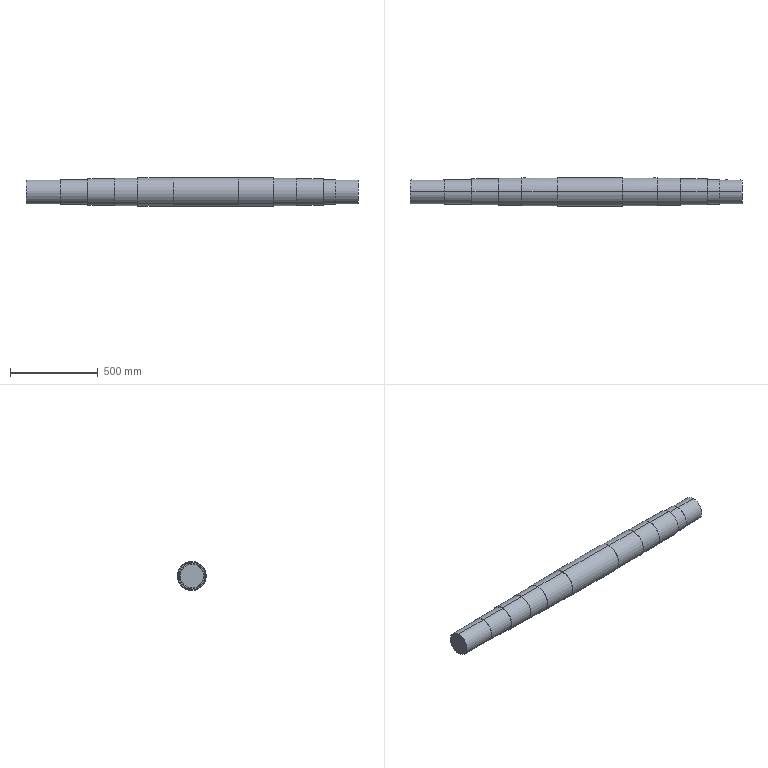Part | NX | features MOVE_FACE 3, BREP 1 | 1 solid | 50 faces | box 1889 x 162.539 x 165 mm | volume 34030029 mm3 | cylinder 29 | plane 21 | commonest cylinder face diameters 36 x4 135 x4 140 x4 150 x4 155 x4 160 x4
STEP:
#1=CARTESIAN_POINT('',(670.,0.,-70.));
#2=VERTEX_POINT('',#1);
#3=CARTESIAN_POINT('',(670.,0.,70.));
#4=VERTEX_POINT('',#3);
#5=CARTESIAN_POINT('',(670.,0.,0.));
#6=DIRECTION('',(1.,0.,0.));
#7=DIRECTION('',(0.,0.,-1.));
#8=AXIS2_PLACEMENT_3D('',#5,#6,#7);
#9=CIRCLE('',#8,70.);
#10=EDGE_CURVE('',#2,#4,#9,.T.);
#11=ORIENTED_EDGE('',*,*,#10,.T.);
#12=CARTESIAN_POINT('',(740.,0.,70.));
#13=VERTEX_POINT('',#12);
#14=CARTESIAN_POINT('',(1022.,0.,70.));
#15=DIRECTION('',(1.,0.,0.));
#16=VECTOR('',#15,1000.);
#17=LINE('',#14,#16);
#18=EDGE_CURVE('',#13,#4,#17,.F.);
#19=ORIENTED_EDGE('',*,*,#18,.F.);
#20=CARTESIAN_POINT('',(740.,0.,-70.));
#21=VERTEX_POINT('',#20);
#22=CARTESIAN_POINT('',(740.,0.,0.));
#23=DIRECTION('',(1.,0.,0.));
#24=DIRECTION('',(0.,0.,-1.));
#25=AXIS2_PLACEMENT_3D('',#22,#23,#24);
#26=CIRCLE('',#25,70.);
#27=EDGE_CURVE('',#21,#13,#26,.T.);
#28=ORIENTED_EDGE('',*,*,#27,.F.);
#29=CARTESIAN_POINT('',(1022.,0.,-70.));
#30=DIRECTION('',(1.,0.,0.));
#31=VECTOR('',#30,1000.);
#32=LINE('',#29,#31);
#33=EDGE_CURVE('',#21,#2,#32,.F.);
#34=ORIENTED_EDGE('',*,*,#33,.T.);
#35=EDGE_LOOP('',(#11,#19,#28,#34));
#36=FACE_BOUND('',#35,.T.);
#37=CARTESIAN_POINT('',(1022.,0.,0.));
#38=DIRECTION('',(1.,0.,0.));
#39=DIRECTION('',(0.,0.,1.));
#40=AXIS2_PLACEMENT_3D('',#37,#38,#39);
#41=CYLINDRICAL_SURFACE('',#40,70.);
#42=ADVANCED_FACE('',(#36),#41,.T.);
#43=CARTESIAN_POINT('',(517.,0.,-75.));
#44=VERTEX_POINT('',#43);
#45=CARTESIAN_POINT('',(517.,0.,75.));
#46=VERTEX_POINT('',#45);
#47=CARTESIAN_POINT('',(517.,0.,0.));
#48=DIRECTION('',(1.,0.,0.));
#49=DIRECTION('',(0.,0.,-1.));
#50=AXIS2_PLACEMENT_3D('',#47,#48,#49);
#51=CIRCLE('',#50,75.);
#52=EDGE_CURVE('',#44,#46,#51,.T.);
#53=ORIENTED_EDGE('',*,*,#52,.T.);
#54=CARTESIAN_POINT('',(670.,0.,75.));
#55=VERTEX_POINT('',#54);
#56=CARTESIAN_POINT('',(1022.,0.,75.));
#57=DIRECTION('',(1.,0.,0.));
#58=VECTOR('',#57,1000.);
#59=LINE('',#56,#58);
#60=EDGE_CURVE('',#55,#46,#59,.F.);
#61=ORIENTED_EDGE('',*,*,#60,.F.);
#62=CARTESIAN_POINT('',(670.,0.,-75.));
#63=VERTEX_POINT('',#62);
#64=CARTESIAN_POINT('',(670.,0.,0.));
#65=DIRECTION('',(1.,0.,0.));
#66=DIRECTION('',(0.,0.,-1.));
#67=AXIS2_PLACEMENT_3D('',#64,#65,#66);
#68=CIRCLE('',#67,75.);
#69=EDGE_CURVE('',#63,#55,#68,.T.);
#70=ORIENTED_EDGE('',*,*,#69,.F.);
#71=CARTESIAN_POINT('',(1022.,0.,-75.));
#72=DIRECTION('',(1.,0.,0.));
#73=VECTOR('',#72,1000.);
#74=LINE('',#71,#73);
#75=EDGE_CURVE('',#63,#44,#74,.F.);
#76=ORIENTED_EDGE('',*,*,#75,.T.);
#77=EDGE_LOOP('',(#53,#61,#70,#76));
#78=FACE_BOUND('',#77,.T.);
#79=CARTESIAN_POINT('',(1022.,0.,0.));
#80=DIRECTION('',(1.,0.,0.));
#81=DIRECTION('',(0.,0.,1.));
#82=AXIS2_PLACEMENT_3D('',#79,#80,#81);
#83=CYLINDRICAL_SURFACE('',#82,75.);
#84=ADVANCED_FACE('',(#78),#83,.T.);
#85=CARTESIAN_POINT('',(385.,0.,-77.5));
#86=VERTEX_POINT('',#85);
#87=CARTESIAN_POINT('',(385.,0.,77.5));
#88=VERTEX_POINT('',#87);
#89=CARTESIAN_POINT('',(385.,0.,0.));
#90=DIRECTION('',(1.,0.,0.));
#91=DIRECTION('',(0.,0.,-1.));
#92=AXIS2_PLACEMENT_3D('',#89,#90,#91);
#93=CIRCLE('',#92,77.5);
#94=EDGE_CURVE('',#86,#88,#93,.T.);
#95=ORIENTED_EDGE('',*,*,#94,.T.);
#96=CARTESIAN_POINT('',(517.,0.,77.5));
#97=VERTEX_POINT('',#96);
#98=CARTESIAN_POINT('',(1022.,0.,77.5));
#99=DIRECTION('',(1.,0.,0.));
#100=VECTOR('',#99,1000.);
#101=LINE('',#98,#100);
#102=EDGE_CURVE('',#97,#88,#101,.F.);
#103=ORIENTED_EDGE('',*,*,#102,.F.);
#104=CARTESIAN_POINT('',(517.,0.,-77.5));
#105=VERTEX_POINT('',#104);
#106=CARTESIAN_POINT('',(517.,0.,0.));
#107=DIRECTION('',(1.,0.,0.));
#108=DIRECTION('',(0.,0.,-1.));
#109=AXIS2_PLACEMENT_3D('',#106,#107,#108);
#110=CIRCLE('',#109,77.5);
#111=EDGE_CURVE('',#105,#97,#110,.T.);
#112=ORIENTED_EDGE('',*,*,#111,.F.);
#113=CARTESIAN_POINT('',(1022.,0.,-77.5));
#114=DIRECTION('',(1.,0.,0.));
#115=VECTOR('',#114,1000.);
#116=LINE('',#113,#115);
#117=EDGE_CURVE('',#105,#86,#116,.F.);
#118=ORIENTED_EDGE('',*,*,#117,.T.);
#119=EDGE_LOOP('',(#95,#103,#112,#118));
#120=FACE_BOUND('',#119,.T.);
#121=CARTESIAN_POINT('',(1022.,0.,0.));
#122=DIRECTION('',(1.,0.,0.));
#123=DIRECTION('',(0.,0.,1.));
#124=AXIS2_PLACEMENT_3D('',#121,#122,#123);
#125=CYLINDRICAL_SURFACE('',#124,77.5);
#126=ADVANCED_FACE('',(#120),#125,.T.);
#127=CARTESIAN_POINT('',(-517.,0.,-77.5));
#128=VERTEX_POINT('',#127);
#129=CARTESIAN_POINT('',(-517.,0.,77.5));
#130=VERTEX_POINT('',#129);
#131=CARTESIAN_POINT('',(-517.,0.,0.));
#132=DIRECTION('',(1.,0.,0.));
#133=DIRECTION('',(0.,0.,-1.));
#134=AXIS2_PLACEMENT_3D('',#131,#132,#133);
#135=CIRCLE('',#134,77.5);
#136=EDGE_CURVE('',#128,#130,#135,.T.);
#137=ORIENTED_EDGE('',*,*,#136,.T.);
#138=CARTESIAN_POINT('',(-385.,0.,77.5));
#139=VERTEX_POINT('',#138);
#140=CARTESIAN_POINT('',(1022.,0.,77.5));
#141=DIRECTION('',(1.,0.,0.));
#142=VECTOR('',#141,1000.);
#143=LINE('',#140,#142);
#144=EDGE_CURVE('',#139,#130,#143,.F.);
#145=ORIENTED_EDGE('',*,*,#144,.F.);
#146=CARTESIAN_POINT('',(-385.,0.,-77.5));
#147=VERTEX_POINT('',#146);
#148=CARTESIAN_POINT('',(-385.,0.,0.));
#149=DIRECTION('',(1.,0.,0.));
#150=DIRECTION('',(0.,0.,-1.));
#151=AXIS2_PLACEMENT_3D('',#148,#149,#150);
#152=CIRCLE('',#151,77.5);
#153=EDGE_CURVE('',#147,#139,#152,.T.);
#154=ORIENTED_EDGE('',*,*,#153,.F.);
#155=CARTESIAN_POINT('',(1022.,0.,-77.5));
#156=DIRECTION('',(1.,0.,0.));
#157=VECTOR('',#156,1000.);
#158=LINE('',#155,#157);
#159=EDGE_CURVE('',#147,#128,#158,.F.);
#160=ORIENTED_EDGE('',*,*,#159,.T.);
#161=EDGE_LOOP('',(#137,#145,#154,#160));
#162=FACE_BOUND('',#161,.T.);
#163=CARTESIAN_POINT('',(1022.,0.,0.));
#164=DIRECTION('',(1.,0.,0.));
#165=DIRECTION('',(0.,0.,1.));
#166=AXIS2_PLACEMENT_3D('',#163,#164,#165);
#167=CYLINDRICAL_SURFACE('',#166,77.5);
#168=ADVANCED_FACE('',(#162),#167,.T.);
#169=CARTESIAN_POINT('',(-670.,0.,-75.));
#170=VERTEX_POINT('',#169);
#171=CARTESIAN_POINT('',(-670.,0.,75.));
#172=VERTEX_POINT('',#171);
#173=CARTESIAN_POINT('',(-670.,0.,0.));
#174=DIRECTION('',(1.,0.,0.));
#175=DIRECTION('',(0.,0.,-1.));
#176=AXIS2_PLACEMENT_3D('',#173,#174,#175);
#177=CIRCLE('',#176,75.);
#178=EDGE_CURVE('',#170,#172,#177,.T.);
#179=ORIENTED_EDGE('',*,*,#178,.T.);
#180=CARTESIAN_POINT('',(-517.,0.,75.));
#181=VERTEX_POINT('',#180);
#182=CARTESIAN_POINT('',(1022.,0.,75.));
#183=DIRECTION('',(1.,0.,0.));
#184=VECTOR('',#183,1000.);
#185=LINE('',#182,#184);
#186=EDGE_CURVE('',#181,#172,#185,.F.);
#187=ORIENTED_EDGE('',*,*,#186,.F.);
#188=CARTESIAN_POINT('',(-517.,0.,-75.));
#189=VERTEX_POINT('',#188);
#190=CARTESIAN_POINT('',(-517.,0.,0.));
#191=DIRECTION('',(1.,0.,0.));
#192=DIRECTION('',(0.,0.,-1.));
#193=AXIS2_PLACEMENT_3D('',#190,#191,#192);
#194=CIRCLE('',#193,75.);
#195=EDGE_CURVE('',#189,#181,#194,.T.);
#196=ORIENTED_EDGE('',*,*,#195,.F.);
#197=CARTESIAN_POINT('',(1022.,0.,-75.));
#198=DIRECTION('',(1.,0.,0.));
#199=VECTOR('',#198,1000.);
#200=LINE('',#197,#199);
#201=EDGE_CURVE('',#189,#170,#200,.F.);
#202=ORIENTED_EDGE('',*,*,#201,.T.);
#203=EDGE_LOOP('',(#179,#187,#196,#202));
#204=FACE_BOUND('',#203,.T.);
#205=CARTESIAN_POINT('',(1022.,0.,0.));
#206=DIRECTION('',(1.,0.,0.));
#207=DIRECTION('',(0.,0.,1.));
#208=AXIS2_PLACEMENT_3D('',#205,#206,#207);
#209=CYLINDRICAL_SURFACE('',#208,75.);
#210=ADVANCED_FACE('',(#204),#209,.T.);
#211=CARTESIAN_POINT('',(-825.,0.,-70.));
#212=VERTEX_POINT('',#211);
#213=CARTESIAN_POINT('',(-825.,0.,70.));
#214=VERTEX_POINT('',#213);
#215=CARTESIAN_POINT('',(-825.,0.,0.));
#216=DIRECTION('',(1.,0.,0.));
#217=DIRECTION('',(0.,0.,-1.));
#218=AXIS2_PLACEMENT_3D('',#215,#216,#217);
#219=CIRCLE('',#218,70.);
#220=EDGE_CURVE('',#212,#214,#219,.T.);
#221=ORIENTED_EDGE('',*,*,#220,.T.);
#222=CARTESIAN_POINT('',(-670.,0.,70.));
#223=VERTEX_POINT('',#222);
#224=CARTESIAN_POINT('',(1022.,0.,70.));
#225=DIRECTION('',(1.,0.,0.));
#226=VECTOR('',#225,1000.);
#227=LINE('',#224,#226);
#228=EDGE_CURVE('',#223,#214,#227,.F.);
#229=ORIENTED_EDGE('',*,*,#228,.F.);
#230=CARTESIAN_POINT('',(-670.,0.,-70.));
#231=VERTEX_POINT('',#230);
#232=CARTESIAN_POINT('',(-670.,0.,0.));
#233=DIRECTION('',(1.,0.,0.));
#234=DIRECTION('',(0.,0.,-1.));
#235=AXIS2_PLACEMENT_3D('',#232,#233,#234);
#236=CIRCLE('',#235,70.);
#237=EDGE_CURVE('',#231,#223,#236,.T.);
#238=ORIENTED_EDGE('',*,*,#237,.F.);
#239=CARTESIAN_POINT('',(1022.,0.,-70.));
#240=DIRECTION('',(1.,0.,0.));
#241=VECTOR('',#240,1000.);
#242=LINE('',#239,#241);
#243=EDGE_CURVE('',#231,#212,#242,.F.);
#244=ORIENTED_EDGE('',*,*,#243,.T.);
#245=EDGE_LOOP('',(#221,#229,#238,#244));
#246=FACE_BOUND('',#245,.T.);
#247=CARTESIAN_POINT('',(1022.,0.,0.));
#248=DIRECTION('',(1.,0.,0.));
#249=DIRECTION('',(0.,0.,1.));
#250=AXIS2_PLACEMENT_3D('',#247,#248,#249);
#251=CYLINDRICAL_SURFACE('',#250,70.);
#252=ADVANCED_FACE('',(#246),#251,.T.);
#253=CARTESIAN_POINT('',(-850.,65.056,18.));
#254=VERTEX_POINT('',#253);
#255=CARTESIAN_POINT('',(-850.,65.056,-18.));
#256=VERTEX_POINT('',#255);
#257=CARTESIAN_POINT('',(-850.,65.056,18.));
#258=CARTESIAN_POINT('',(-847.61,65.056,18.));
#259=CARTESIAN_POINT('',(-842.909,65.33,17.049));
#260=CARTESIAN_POINT('',(-836.943,66.292,13.054));
#261=CARTESIAN_POINT('',(-832.954,67.237,7.104));
#262=CARTESIAN_POINT('',(-831.526,67.63,0.01848));
#263=CARTESIAN_POINT('',(-832.942,67.242,-7.078));
#264=CARTESIAN_POINT('',(-838.272,65.966,-15.054));
#265=CARTESIAN_POINT('',(-845.221,65.056,-18.));
#266=CARTESIAN_POINT('',(-850.,65.056,-18.));
#267=B_SPLINE_CURVE_WITH_KNOTS('',3,(#257,#258,#259,#260,#261,#262,#263,#264,#265,#266),.UNSPECIFIED.,.F.,.F.,(4,1,1,1,1,1,1,4),(0.,0.007064,0.01413,0.02119,0.02826,0.03532,0.04239,0.05651),.UNSPECIFIED.);
#268=EDGE_CURVE('',#254,#256,#267,.T.);
#269=ORIENTED_EDGE('',*,*,#268,.F.);
#270=CARTESIAN_POINT('',(-994.,65.056,18.));
#271=VERTEX_POINT('',#270);
#272=CARTESIAN_POINT('',(1022.,65.056,18.));
#273=DIRECTION('',(1.,0.,0.));
#274=VECTOR('',#273,1000.);
#275=LINE('',#272,#274);
#276=EDGE_CURVE('',#271,#254,#275,.T.);
#277=ORIENTED_EDGE('',*,*,#276,.F.);
#278=CARTESIAN_POINT('',(-994.,65.056,-18.));
#279=VERTEX_POINT('',#278);
#280=CARTESIAN_POINT('',(-994.,65.056,-18.));
#281=CARTESIAN_POINT('',(-996.39,65.056,-18.));
#282=CARTESIAN_POINT('',(-1001.091,65.33,-17.049));
#283=CARTESIAN_POINT('',(-1007.057,66.292,-13.054));
#284=CARTESIAN_POINT('',(-1011.046,67.237,-7.104));
#285=CARTESIAN_POINT('',(-1012.474,67.63,-0.01848));
#286=CARTESIAN_POINT('',(-1011.058,67.242,7.078));
#287=CARTESIAN_POINT('',(-1005.728,65.966,15.054));
#288=CARTESIAN_POINT('',(-998.779,65.056,18.));
#289=CARTESIAN_POINT('',(-994.,65.056,18.));
#290=B_SPLINE_CURVE_WITH_KNOTS('',3,(#280,#281,#282,#283,#284,#285,#286,#287,#288,#289),.UNSPECIFIED.,.F.,.F.,(4,1,1,1,1,1,1,4),(0.,0.007064,0.01413,0.02119,0.02826,0.03532,0.04239,0.05651),.UNSPECIFIED.);
#291=EDGE_CURVE('',#279,#271,#290,.T.);
#292=ORIENTED_EDGE('',*,*,#291,.F.);
#293=CARTESIAN_POINT('',(1022.,65.056,-18.));
#294=DIRECTION('',(-1.,0.,0.));
#295=VECTOR('',#294,1000.);
#296=LINE('',#293,#295);
#297=EDGE_CURVE('',#256,#279,#296,.T.);
#298=ORIENTED_EDGE('',*,*,#297,.F.);
#299=EDGE_LOOP('',(#269,#277,#292,#298));
#300=FACE_BOUND('',#299,.T.);
#301=CARTESIAN_POINT('',(-1022.,0.,-67.5));
#302=VERTEX_POINT('',#301);
#303=CARTESIAN_POINT('',(-1022.,0.,67.5));
#304=VERTEX_POINT('',#303);
#305=CARTESIAN_POINT('',(-1022.,0.,0.));
#306=DIRECTION('',(1.,0.,0.));
#307=DIRECTION('',(0.,0.,-1.));
#308=AXIS2_PLACEMENT_3D('',#305,#306,#307);
#309=CIRCLE('',#308,67.5);
#310=EDGE_CURVE('',#302,#304,#309,.T.);
#311=ORIENTED_EDGE('',*,*,#310,.T.);
#312=CARTESIAN_POINT('',(-825.,0.,67.5));
#313=VERTEX_POINT('',#312);
#314=CARTESIAN_POINT('',(1022.,0.,67.5));
#315=DIRECTION('',(1.,0.,0.));
#316=VECTOR('',#315,1000.);
#317=LINE('',#314,#316);
#318=EDGE_CURVE('',#313,#304,#317,.F.);
#319=ORIENTED_EDGE('',*,*,#318,.F.);
#320=CARTESIAN_POINT('',(-825.,0.,-67.5));
#321=VERTEX_POINT('',#320);
#322=CARTESIAN_POINT('',(-825.,0.,0.));
#323=DIRECTION('',(1.,0.,0.));
#324=DIRECTION('',(0.,0.,-1.));
#325=AXIS2_PLACEMENT_3D('',#322,#323,#324);
#326=CIRCLE('',#325,67.5);
#327=EDGE_CURVE('',#321,#313,#326,.T.);
#328=ORIENTED_EDGE('',*,*,#327,.F.);
#329=CARTESIAN_POINT('',(1022.,0.,-67.5));
#330=DIRECTION('',(1.,0.,0.));
#331=VECTOR('',#330,1000.);
#332=LINE('',#329,#331);
#333=EDGE_CURVE('',#321,#302,#332,.F.);
#334=ORIENTED_EDGE('',*,*,#333,.T.);
#335=EDGE_LOOP('',(#311,#319,#328,#334));
#336=FACE_BOUND('',#335,.T.);
#337=CARTESIAN_POINT('',(1022.,0.,0.));
#338=DIRECTION('',(1.,0.,0.));
#339=DIRECTION('',(0.,0.,1.));
#340=AXIS2_PLACEMENT_3D('',#337,#338,#339);
#341=CYLINDRICAL_SURFACE('',#340,67.5);
#342=ADVANCED_FACE('',(#300,#336),#341,.T.);
#343=CARTESIAN_POINT('',(185.,77.46,20.));
#344=VERTEX_POINT('',#343);
#345=CARTESIAN_POINT('',(185.,0.,80.));
#346=VERTEX_POINT('',#345);
#347=CARTESIAN_POINT('',(185.,0.,0.));
#348=DIRECTION('',(1.,0.,0.));
#349=DIRECTION('',(0.,0.,-1.));
#350=AXIS2_PLACEMENT_3D('',#347,#348,#349);
#351=CIRCLE('',#350,80.);
#352=EDGE_CURVE('',#344,#346,#351,.T.);
#353=ORIENTED_EDGE('',*,*,#352,.T.);
#354=CARTESIAN_POINT('',(385.,0.,80.));
#355=VERTEX_POINT('',#354);
#356=CARTESIAN_POINT('',(1022.,0.,80.));
#357=DIRECTION('',(1.,0.,0.));
#358=VECTOR('',#357,1000.);
#359=LINE('',#356,#358);
#360=EDGE_CURVE('',#355,#346,#359,.F.);
#361=ORIENTED_EDGE('',*,*,#360,.F.);
#362=CARTESIAN_POINT('',(385.,0.,-80.));
#363=VERTEX_POINT('',#362);
#364=CARTESIAN_POINT('',(385.,0.,0.));
#365=DIRECTION('',(1.,0.,0.));
#366=DIRECTION('',(0.,0.,-1.));
#367=AXIS2_PLACEMENT_3D('',#364,#365,#366);
#368=CIRCLE('',#367,80.);
#369=EDGE_CURVE('',#363,#355,#368,.T.);
#370=ORIENTED_EDGE('',*,*,#369,.F.);
#371=CARTESIAN_POINT('',(185.,0.,-80.));
#372=VERTEX_POINT('',#371);
#373=CARTESIAN_POINT('',(1022.,0.,-80.));
#374=DIRECTION('',(1.,0.,0.));
#375=VECTOR('',#374,1000.);
#376=LINE('',#373,#375);
#377=EDGE_CURVE('',#363,#372,#376,.F.);
#378=ORIENTED_EDGE('',*,*,#377,.T.);
#379=CARTESIAN_POINT('',(185.,77.46,-20.));
#380=VERTEX_POINT('',#379);
#381=CARTESIAN_POINT('',(185.,0.,0.));
#382=DIRECTION('',(1.,0.,0.));
#383=DIRECTION('',(0.,0.,-1.));
#384=AXIS2_PLACEMENT_3D('',#381,#382,#383);
#385=CIRCLE('',#384,80.);
#386=EDGE_CURVE('',#372,#380,#385,.T.);
#387=ORIENTED_EDGE('',*,*,#386,.T.);
#388=CARTESIAN_POINT('',(350.,77.46,-20.));
#389=VERTEX_POINT('',#388);
#390=CARTESIAN_POINT('',(1022.,77.46,-20.));
#391=DIRECTION('',(1.,0.,0.));
#392=VECTOR('',#391,1000.);
#393=LINE('',#390,#392);
#394=EDGE_CURVE('',#380,#389,#393,.T.);
#395=ORIENTED_EDGE('',*,*,#394,.T.);
#396=CARTESIAN_POINT('',(350.,77.46,20.));
#397=VERTEX_POINT('',#396);
#398=CARTESIAN_POINT('',(350.,77.46,-20.));
#399=CARTESIAN_POINT('',(352.653,77.46,-20.));
#400=CARTESIAN_POINT('',(357.875,77.743,-18.945));
#401=CARTESIAN_POINT('',(364.509,78.743,-14.505));
#402=CARTESIAN_POINT('',(368.941,79.726,-7.889));
#403=CARTESIAN_POINT('',(370.526,80.136,-0.02022));
#404=CARTESIAN_POINT('',(368.956,79.729,7.863));
#405=CARTESIAN_POINT('',(364.512,78.743,14.503));
#406=CARTESIAN_POINT('',(357.885,77.744,18.941));
#407=CARTESIAN_POINT('',(352.654,77.46,20.));
#408=CARTESIAN_POINT('',(350.,77.46,20.));
#409=B_SPLINE_CURVE_WITH_KNOTS('',3,(#398,#399,#400,#401,#402,#403,#404,#405,#406,#407,#408),.UNSPECIFIED.,.F.,.F.,(4,1,1,1,1,1,1,1,4),(0.,0.007845,0.01569,0.02353,0.03138,0.03922,0.04707,0.05491,0.06276),.UNSPECIFIED.);
#410=EDGE_CURVE('',#389,#397,#409,.T.);
#411=ORIENTED_EDGE('',*,*,#410,.T.);
#412=CARTESIAN_POINT('',(1022.,77.46,20.));
#413=DIRECTION('',(-1.,0.,0.));
#414=VECTOR('',#413,1000.);
#415=LINE('',#412,#414);
#416=EDGE_CURVE('',#397,#344,#415,.T.);
#417=ORIENTED_EDGE('',*,*,#416,.T.);
#418=EDGE_LOOP('',(#353,#361,#370,#378,#387,#395,#411,#417));
#419=FACE_BOUND('',#418,.T.);
#420=CARTESIAN_POINT('',(1022.,0.,0.));
#421=DIRECTION('',(1.,0.,0.));
#422=DIRECTION('',(0.,0.,1.));
#423=AXIS2_PLACEMENT_3D('',#420,#421,#422);
#424=CYLINDRICAL_SURFACE('',#423,80.);
#425=ADVANCED_FACE('',(#419),#424,.T.);
#426=CARTESIAN_POINT('',(-185.,80.039,20.));
#427=VERTEX_POINT('',#426);
#428=CARTESIAN_POINT('',(-185.,0.,82.5));
#429=VERTEX_POINT('',#428);
#430=CARTESIAN_POINT('',(-185.,0.,0.));
#431=DIRECTION('',(1.,0.,0.));
#432=DIRECTION('',(0.,0.,-1.));
#433=AXIS2_PLACEMENT_3D('',#430,#431,#432);
#434=CIRCLE('',#433,82.5);
#435=EDGE_CURVE('',#427,#429,#434,.T.);
#436=ORIENTED_EDGE('',*,*,#435,.T.);
#437=CARTESIAN_POINT('',(185.,0.,82.5));
#438=VERTEX_POINT('',#437);
#439=CARTESIAN_POINT('',(1022.,0.,82.5));
#440=DIRECTION('',(1.,0.,0.));
#441=VECTOR('',#440,1000.);
#442=LINE('',#439,#441);
#443=EDGE_CURVE('',#429,#438,#442,.T.);
#444=ORIENTED_EDGE('',*,*,#443,.T.);
#445=CARTESIAN_POINT('',(185.,80.039,20.));
#446=VERTEX_POINT('',#445);
#447=CARTESIAN_POINT('',(185.,0.,0.));
#448=DIRECTION('',(1.,0.,0.));
#449=DIRECTION('',(0.,0.,-1.));
#450=AXIS2_PLACEMENT_3D('',#447,#448,#449);
#451=CIRCLE('',#450,82.5);
#452=EDGE_CURVE('',#446,#438,#451,.T.);
#453=ORIENTED_EDGE('',*,*,#452,.F.);
#454=CARTESIAN_POINT('',(1022.,80.039,20.));
#455=DIRECTION('',(-1.,0.,0.));
#456=VECTOR('',#455,1000.);
#457=LINE('',#454,#456);
#458=EDGE_CURVE('',#446,#427,#457,.T.);
#459=ORIENTED_EDGE('',*,*,#458,.T.);
#460=EDGE_LOOP('',(#436,#444,#453,#459));
#461=FACE_BOUND('',#460,.T.);
#462=CARTESIAN_POINT('',(1022.,0.,0.));
#463=DIRECTION('',(1.,0.,0.));
#464=DIRECTION('',(0.,0.,1.));
#465=AXIS2_PLACEMENT_3D('',#462,#463,#464);
#466=CYLINDRICAL_SURFACE('',#465,82.5);
#467=ADVANCED_FACE('',(#461),#466,.T.);
#468=ORIENTED_EDGE('',*,*,#443,.F.);
#469=CARTESIAN_POINT('',(-185.,0.,-82.5));
#470=VERTEX_POINT('',#469);
#471=CARTESIAN_POINT('',(-185.,0.,0.));
#472=DIRECTION('',(1.,0.,0.));
#473=DIRECTION('',(0.,0.,-1.));
#474=AXIS2_PLACEMENT_3D('',#471,#472,#473);
#475=CIRCLE('',#474,82.5);
#476=EDGE_CURVE('',#429,#470,#475,.T.);
#477=ORIENTED_EDGE('',*,*,#476,.T.);
#478=CARTESIAN_POINT('',(185.,0.,-82.5));
#479=VERTEX_POINT('',#478);
#480=CARTESIAN_POINT('',(1022.,0.,-82.5));
#481=DIRECTION('',(1.,0.,0.));
#482=VECTOR('',#481,1000.);
#483=LINE('',#480,#482);
#484=EDGE_CURVE('',#470,#479,#483,.T.);
#485=ORIENTED_EDGE('',*,*,#484,.T.);
#486=CARTESIAN_POINT('',(185.,0.,0.));
#487=DIRECTION('',(1.,0.,0.));
#488=DIRECTION('',(0.,0.,-1.));
#489=AXIS2_PLACEMENT_3D('',#486,#487,#488);
#490=CIRCLE('',#489,82.5);
#491=EDGE_CURVE('',#438,#479,#490,.T.);
#492=ORIENTED_EDGE('',*,*,#491,.F.);
#493=EDGE_LOOP('',(#468,#477,#485,#492));
#494=FACE_BOUND('',#493,.T.);
#495=CARTESIAN_POINT('',(1022.,0.,0.));
#496=DIRECTION('',(1.,0.,0.));
#497=DIRECTION('',(0.,0.,1.));
#498=AXIS2_PLACEMENT_3D('',#495,#496,#497);
#499=CYLINDRICAL_SURFACE('',#498,82.5);
#500=ADVANCED_FACE('',(#494),#499,.T.);
#501=CARTESIAN_POINT('',(-385.,0.,-80.));
#502=VERTEX_POINT('',#501);
#503=CARTESIAN_POINT('',(-385.,0.,80.));
#504=VERTEX_POINT('',#503);
#505=CARTESIAN_POINT('',(-385.,0.,0.));
#506=DIRECTION('',(1.,0.,0.));
#507=DIRECTION('',(0.,0.,-1.));
#508=AXIS2_PLACEMENT_3D('',#505,#506,#507);
#509=CIRCLE('',#508,80.);
#510=EDGE_CURVE('',#502,#504,#509,.T.);
#511=ORIENTED_EDGE('',*,*,#510,.T.);
#512=CARTESIAN_POINT('',(-185.,0.,80.));
#513=VERTEX_POINT('',#512);
#514=CARTESIAN_POINT('',(1022.,0.,80.));
#515=DIRECTION('',(1.,0.,0.));
#516=VECTOR('',#515,1000.);
#517=LINE('',#514,#516);
#518=EDGE_CURVE('',#513,#504,#517,.F.);
#519=ORIENTED_EDGE('',*,*,#518,.F.);
#520=CARTESIAN_POINT('',(-185.,77.46,20.));
#521=VERTEX_POINT('',#520);
#522=CARTESIAN_POINT('',(-185.,0.,0.));
#523=DIRECTION('',(1.,0.,0.));
#524=DIRECTION('',(0.,0.,-1.));
#525=AXIS2_PLACEMENT_3D('',#522,#523,#524);
#526=CIRCLE('',#525,80.);
#527=EDGE_CURVE('',#521,#513,#526,.T.);
#528=ORIENTED_EDGE('',*,*,#527,.F.);
#529=CARTESIAN_POINT('',(-350.,77.46,20.));
#530=VERTEX_POINT('',#529);
#531=CARTESIAN_POINT('',(1022.,77.46,20.));
#532=DIRECTION('',(-1.,0.,0.));
#533=VECTOR('',#532,1000.);
#534=LINE('',#531,#533);
#535=EDGE_CURVE('',#521,#530,#534,.T.);
#536=ORIENTED_EDGE('',*,*,#535,.T.);
#537=CARTESIAN_POINT('',(-350.,77.46,-20.));
#538=VERTEX_POINT('',#537);
#539=CARTESIAN_POINT('',(-350.,77.46,20.));
#540=CARTESIAN_POINT('',(-352.653,77.46,20.));
#541=CARTESIAN_POINT('',(-357.875,77.743,18.945));
#542=CARTESIAN_POINT('',(-364.509,78.743,14.505));
#543=CARTESIAN_POINT('',(-368.941,79.726,7.889));
#544=CARTESIAN_POINT('',(-370.526,80.136,0.02022));
#545=CARTESIAN_POINT('',(-368.956,79.729,-7.863));
#546=CARTESIAN_POINT('',(-364.512,78.743,-14.503));
#547=CARTESIAN_POINT('',(-357.885,77.744,-18.941));
#548=CARTESIAN_POINT('',(-352.654,77.46,-20.));
#549=CARTESIAN_POINT('',(-350.,77.46,-20.));
#550=B_SPLINE_CURVE_WITH_KNOTS('',3,(#539,#540,#541,#542,#543,#544,#545,#546,#547,#548,#549),.UNSPECIFIED.,.F.,.F.,(4,1,1,1,1,1,1,1,4),(0.,0.007845,0.01569,0.02353,0.03138,0.03922,0.04707,0.05491,0.06276),.UNSPECIFIED.);
#551=EDGE_CURVE('',#530,#538,#550,.T.);
#552=ORIENTED_EDGE('',*,*,#551,.T.);
#553=CARTESIAN_POINT('',(-185.,77.46,-20.));
#554=VERTEX_POINT('',#553);
#555=CARTESIAN_POINT('',(1022.,77.46,-20.));
#556=DIRECTION('',(1.,0.,0.));
#557=VECTOR('',#556,1000.);
#558=LINE('',#555,#557);
#559=EDGE_CURVE('',#538,#554,#558,.T.);
#560=ORIENTED_EDGE('',*,*,#559,.T.);
#561=CARTESIAN_POINT('',(-185.,0.,-80.));
#562=VERTEX_POINT('',#561);
#563=CARTESIAN_POINT('',(-185.,0.,0.));
#564=DIRECTION('',(1.,0.,0.));
#565=DIRECTION('',(0.,0.,-1.));
#566=AXIS2_PLACEMENT_3D('',#563,#564,#565);
#567=CIRCLE('',#566,80.);
#568=EDGE_CURVE('',#562,#554,#567,.T.);
#569=ORIENTED_EDGE('',*,*,#568,.F.);
#570=CARTESIAN_POINT('',(1022.,0.,-80.));
#571=DIRECTION('',(1.,0.,0.));
#572=VECTOR('',#571,1000.);
#573=LINE('',#570,#572);
#574=EDGE_CURVE('',#562,#502,#573,.F.);
#575=ORIENTED_EDGE('',*,*,#574,.T.);
#576=EDGE_LOOP('',(#511,#519,#528,#536,#552,#560,#569,#575));
#577=FACE_BOUND('',#576,.T.);
#578=CARTESIAN_POINT('',(1022.,0.,0.));
#579=DIRECTION('',(1.,0.,0.));
#580=DIRECTION('',(0.,0.,1.));
#581=AXIS2_PLACEMENT_3D('',#578,#579,#580);
#582=CYLINDRICAL_SURFACE('',#581,80.);
#583=ADVANCED_FACE('',(#577),#582,.T.);
#584=CARTESIAN_POINT('',(839.,65.056,18.));
#585=VERTEX_POINT('',#584);
#586=CARTESIAN_POINT('',(801.,65.056,18.));
#587=VERTEX_POINT('',#586);
#588=CARTESIAN_POINT('',(937.,65.056,18.));
#589=DIRECTION('',(-1.,0.,0.));
#590=VECTOR('',#589,1000.);
#591=LINE('',#588,#590);
#592=EDGE_CURVE('',#585,#587,#591,.T.);
#593=ORIENTED_EDGE('',*,*,#592,.T.);
#594=CARTESIAN_POINT('',(801.,65.056,-18.));
#595=VERTEX_POINT('',#594);
#596=CARTESIAN_POINT('',(801.,65.056,18.));
#597=CARTESIAN_POINT('',(798.61,65.056,18.));
#598=CARTESIAN_POINT('',(793.909,65.33,17.049));
#599=CARTESIAN_POINT('',(787.943,66.292,13.054));
#600=CARTESIAN_POINT('',(783.954,67.237,7.104));
#601=CARTESIAN_POINT('',(782.526,67.63,0.01848));
#602=CARTESIAN_POINT('',(783.942,67.242,-7.078));
#603=CARTESIAN_POINT('',(789.272,65.966,-15.054));
#604=CARTESIAN_POINT('',(796.221,65.056,-18.));
#605=CARTESIAN_POINT('',(801.,65.056,-18.));
#606=B_SPLINE_CURVE_WITH_KNOTS('',3,(#596,#597,#598,#599,#600,#601,#602,#603,#604,#605),.UNSPECIFIED.,.F.,.F.,(4,1,1,1,1,1,1,4),(0.,0.007064,0.01413,0.02119,0.02826,0.03532,0.04239,0.05651),.UNSPECIFIED.);
#607=EDGE_CURVE('',#587,#595,#606,.T.);
#608=ORIENTED_EDGE('',*,*,#607,.T.);
#609=CARTESIAN_POINT('',(839.,65.056,-18.));
#610=VERTEX_POINT('',#609);
#611=CARTESIAN_POINT('',(937.,65.056,-18.));
#612=DIRECTION('',(1.,0.,0.));
#613=VECTOR('',#612,1000.);
#614=LINE('',#611,#613);
#615=EDGE_CURVE('',#595,#610,#614,.T.);
#616=ORIENTED_EDGE('',*,*,#615,.T.);
#617=CARTESIAN_POINT('',(839.,65.056,-18.));
#618=CARTESIAN_POINT('',(841.39,65.056,-18.));
#619=CARTESIAN_POINT('',(846.091,65.33,-17.049));
#620=CARTESIAN_POINT('',(852.057,66.292,-13.054));
#621=CARTESIAN_POINT('',(856.046,67.237,-7.104));
#622=CARTESIAN_POINT('',(857.474,67.63,-0.01848));
#623=CARTESIAN_POINT('',(856.058,67.242,7.078));
#624=CARTESIAN_POINT('',(850.728,65.966,15.054));
#625=CARTESIAN_POINT('',(843.779,65.056,18.));
#626=CARTESIAN_POINT('',(839.,65.056,18.));
#627=B_SPLINE_CURVE_WITH_KNOTS('',3,(#617,#618,#619,#620,#621,#622,#623,#624,#625,#626),.UNSPECIFIED.,.F.,.F.,(4,1,1,1,1,1,1,4),(0.,0.007064,0.01413,0.02119,0.02826,0.03532,0.04239,0.05651),.UNSPECIFIED.);
#628=EDGE_CURVE('',#610,#585,#627,.T.);
#629=ORIENTED_EDGE('',*,*,#628,.T.);
#630=EDGE_LOOP('',(#593,#608,#616,#629));
#631=FACE_BOUND('',#630,.T.);
#632=CARTESIAN_POINT('',(740.,0.,-67.5));
#633=VERTEX_POINT('',#632);
#634=CARTESIAN_POINT('',(740.,0.,67.5));
#635=VERTEX_POINT('',#634);
#636=CARTESIAN_POINT('',(740.,0.,0.));
#637=DIRECTION('',(1.,0.,0.));
#638=DIRECTION('',(0.,0.,-1.));
#639=AXIS2_PLACEMENT_3D('',#636,#637,#638);
#640=CIRCLE('',#639,67.5);
#641=EDGE_CURVE('',#633,#635,#640,.T.);
#642=ORIENTED_EDGE('',*,*,#641,.T.);
#643=CARTESIAN_POINT('',(867.,0.,67.5));
#644=VERTEX_POINT('',#643);
#645=CARTESIAN_POINT('',(937.,0.,67.5));
#646=DIRECTION('',(1.,0.,0.));
#647=VECTOR('',#646,1000.);
#648=LINE('',#645,#647);
#649=EDGE_CURVE('',#644,#635,#648,.F.);
#650=ORIENTED_EDGE('',*,*,#649,.F.);
#651=CARTESIAN_POINT('',(867.,0.,-67.5));
#652=VERTEX_POINT('',#651);
#653=CARTESIAN_POINT('',(867.,0.,0.));
#654=DIRECTION('',(1.,0.,0.));
#655=DIRECTION('',(0.,0.,-1.));
#656=AXIS2_PLACEMENT_3D('',#653,#654,#655);
#657=CIRCLE('',#656,67.5);
#658=EDGE_CURVE('',#652,#644,#657,.T.);
#659=ORIENTED_EDGE('',*,*,#658,.F.);
#660=CARTESIAN_POINT('',(937.,0.,-67.5));
#661=DIRECTION('',(1.,0.,0.));
#662=VECTOR('',#661,1000.);
#663=LINE('',#660,#662);
#664=EDGE_CURVE('',#652,#633,#663,.F.);
#665=ORIENTED_EDGE('',*,*,#664,.T.);
#666=EDGE_LOOP('',(#642,#650,#659,#665));
#667=FACE_BOUND('',#666,.T.);
#668=CARTESIAN_POINT('',(937.,0.,0.));
#669=DIRECTION('',(1.,0.,0.));
#670=DIRECTION('',(0.,0.,1.));
#671=AXIS2_PLACEMENT_3D('',#668,#669,#670);
#672=CYLINDRICAL_SURFACE('',#671,67.5);
#673=ADVANCED_FACE('',(#631,#667),#672,.T.);
#674=ORIENTED_EDGE('',*,*,#649,.T.);
#675=CARTESIAN_POINT('',(740.,0.,0.));
#676=DIRECTION('',(1.,0.,0.));
#677=DIRECTION('',(0.,0.,-1.));
#678=AXIS2_PLACEMENT_3D('',#675,#676,#677);
#679=CIRCLE('',#678,67.5);
#680=EDGE_CURVE('',#635,#633,#679,.T.);
#681=ORIENTED_EDGE('',*,*,#680,.T.);
#682=ORIENTED_EDGE('',*,*,#664,.F.);
#683=CARTESIAN_POINT('',(867.,0.,0.));
#684=DIRECTION('',(1.,0.,0.));
#685=DIRECTION('',(0.,0.,-1.));
#686=AXIS2_PLACEMENT_3D('',#683,#684,#685);
#687=CIRCLE('',#686,67.5);
#688=EDGE_CURVE('',#644,#652,#687,.T.);
#689=ORIENTED_EDGE('',*,*,#688,.F.);
#690=EDGE_LOOP('',(#674,#681,#682,#689));
#691=FACE_BOUND('',#690,.T.);
#692=CARTESIAN_POINT('',(937.,0.,0.));
#693=DIRECTION('',(1.,0.,0.));
#694=DIRECTION('',(0.,0.,1.));
#695=AXIS2_PLACEMENT_3D('',#692,#693,#694);
#696=CYLINDRICAL_SURFACE('',#695,67.5);
#697=ADVANCED_FACE('',(#691),#696,.T.);
#698=ORIENTED_EDGE('',*,*,#518,.T.);
#699=CARTESIAN_POINT('',(-385.,0.,0.));
#700=DIRECTION('',(1.,0.,0.));
#701=DIRECTION('',(0.,0.,-1.));
#702=AXIS2_PLACEMENT_3D('',#699,#700,#701);
#703=CIRCLE('',#702,80.);
#704=EDGE_CURVE('',#504,#502,#703,.T.);
#705=ORIENTED_EDGE('',*,*,#704,.T.);
#706=ORIENTED_EDGE('',*,*,#574,.F.);
#707=CARTESIAN_POINT('',(-185.,0.,0.));
#708=DIRECTION('',(1.,0.,0.));
#709=DIRECTION('',(0.,0.,-1.));
#710=AXIS2_PLACEMENT_3D('',#707,#708,#709);
#711=CIRCLE('',#710,80.);
#712=EDGE_CURVE('',#513,#562,#711,.T.);
#713=ORIENTED_EDGE('',*,*,#712,.F.);
#714=EDGE_LOOP('',(#698,#705,#706,#713));
#715=FACE_BOUND('',#714,.T.);
#716=CARTESIAN_POINT('',(1022.,0.,0.));
#717=DIRECTION('',(1.,0.,0.));
#718=DIRECTION('',(0.,0.,1.));
#719=AXIS2_PLACEMENT_3D('',#716,#717,#718);
#720=CYLINDRICAL_SURFACE('',#719,80.);
#721=ADVANCED_FACE('',(#715),#720,.T.);
#722=ORIENTED_EDGE('',*,*,#435,.F.);
#723=CARTESIAN_POINT('',(-185.,82.5,20.));
#724=DIRECTION('',(0.,-1.,0.));
#725=VECTOR('',#724,1000.);
#726=LINE('',#723,#725);
#727=EDGE_CURVE('',#427,#521,#726,.T.);
#728=ORIENTED_EDGE('',*,*,#727,.T.);
#729=ORIENTED_EDGE('',*,*,#527,.T.);
#730=ORIENTED_EDGE('',*,*,#712,.T.);
#731=ORIENTED_EDGE('',*,*,#568,.T.);
#732=CARTESIAN_POINT('',(-185.,80.039,-20.));
#733=VERTEX_POINT('',#732);
#734=CARTESIAN_POINT('',(-185.,82.5,-20.));
#735=DIRECTION('',(0.,1.,0.));
#736=VECTOR('',#735,1000.);
#737=LINE('',#734,#736);
#738=EDGE_CURVE('',#554,#733,#737,.T.);
#739=ORIENTED_EDGE('',*,*,#738,.T.);
#740=CARTESIAN_POINT('',(-185.,0.,0.));
#741=DIRECTION('',(1.,0.,0.));
#742=DIRECTION('',(0.,0.,-1.));
#743=AXIS2_PLACEMENT_3D('',#740,#741,#742);
#744=CIRCLE('',#743,82.5);
#745=EDGE_CURVE('',#470,#733,#744,.T.);
#746=ORIENTED_EDGE('',*,*,#745,.F.);
#747=ORIENTED_EDGE('',*,*,#476,.F.);
#748=EDGE_LOOP('',(#722,#728,#729,#730,#731,#739,#746,#747));
#749=FACE_BOUND('',#748,.T.);
#750=CARTESIAN_POINT('',(-185.,82.5,0.));
#751=DIRECTION('',(-1.,0.,0.));
#752=DIRECTION('',(0.,0.,-1.));
#753=AXIS2_PLACEMENT_3D('',#750,#751,#752);
#754=PLANE('',#753);
#755=ADVANCED_FACE('',(#749),#754,.T.);
#756=ORIENTED_EDGE('',*,*,#484,.F.);
#757=ORIENTED_EDGE('',*,*,#745,.T.);
#758=CARTESIAN_POINT('',(185.,80.039,-20.));
#759=VERTEX_POINT('',#758);
#760=CARTESIAN_POINT('',(1022.,80.039,-20.));
#761=DIRECTION('',(1.,0.,0.));
#762=VECTOR('',#761,1000.);
#763=LINE('',#760,#762);
#764=EDGE_CURVE('',#733,#759,#763,.T.);
#765=ORIENTED_EDGE('',*,*,#764,.T.);
#766=CARTESIAN_POINT('',(185.,0.,0.));
#767=DIRECTION('',(1.,0.,0.));
#768=DIRECTION('',(0.,0.,-1.));
#769=AXIS2_PLACEMENT_3D('',#766,#767,#768);
#770=CIRCLE('',#769,82.5);
#771=EDGE_CURVE('',#479,#759,#770,.T.);
#772=ORIENTED_EDGE('',*,*,#771,.F.);
#773=EDGE_LOOP('',(#756,#757,#765,#772));
#774=FACE_BOUND('',#773,.T.);
#775=CARTESIAN_POINT('',(1022.,0.,0.));
#776=DIRECTION('',(1.,0.,0.));
#777=DIRECTION('',(0.,0.,1.));
#778=AXIS2_PLACEMENT_3D('',#775,#776,#777);
#779=CYLINDRICAL_SURFACE('',#778,82.5);
#780=ADVANCED_FACE('',(#774),#779,.T.);
#781=ORIENTED_EDGE('',*,*,#352,.F.);
#782=CARTESIAN_POINT('',(185.,82.5,20.));
#783=DIRECTION('',(0.,1.,0.));
#784=VECTOR('',#783,1000.);
#785=LINE('',#782,#784);
#786=EDGE_CURVE('',#344,#446,#785,.T.);
#787=ORIENTED_EDGE('',*,*,#786,.T.);
#788=ORIENTED_EDGE('',*,*,#452,.T.);
#789=ORIENTED_EDGE('',*,*,#491,.T.);
#790=ORIENTED_EDGE('',*,*,#771,.T.);
#791=CARTESIAN_POINT('',(185.,82.5,-20.));
#792=DIRECTION('',(0.,-1.,0.));
#793=VECTOR('',#792,1000.);
#794=LINE('',#791,#793);
#795=EDGE_CURVE('',#759,#380,#794,.T.);
#796=ORIENTED_EDGE('',*,*,#795,.T.);
#797=ORIENTED_EDGE('',*,*,#386,.F.);
#798=CARTESIAN_POINT('',(185.,0.,0.));
#799=DIRECTION('',(1.,0.,0.));
#800=DIRECTION('',(0.,0.,-1.));
#801=AXIS2_PLACEMENT_3D('',#798,#799,#800);
#802=CIRCLE('',#801,80.);
#803=EDGE_CURVE('',#346,#372,#802,.T.);
#804=ORIENTED_EDGE('',*,*,#803,.F.);
#805=EDGE_LOOP('',(#781,#787,#788,#789,#790,#796,#797,#804));
#806=FACE_BOUND('',#805,.T.);
#807=CARTESIAN_POINT('',(185.,82.5,0.));
#808=DIRECTION('',(1.,0.,0.));
#809=DIRECTION('',(0.,0.,1.));
#810=AXIS2_PLACEMENT_3D('',#807,#808,#809);
#811=PLANE('',#810);
#812=ADVANCED_FACE('',(#806),#811,.T.);
#813=ORIENTED_EDGE('',*,*,#360,.T.);
#814=ORIENTED_EDGE('',*,*,#803,.T.);
#815=ORIENTED_EDGE('',*,*,#377,.F.);
#816=CARTESIAN_POINT('',(385.,0.,0.));
#817=DIRECTION('',(1.,0.,0.));
#818=DIRECTION('',(0.,0.,-1.));
#819=AXIS2_PLACEMENT_3D('',#816,#817,#818);
#820=CIRCLE('',#819,80.);
#821=EDGE_CURVE('',#355,#363,#820,.T.);
#822=ORIENTED_EDGE('',*,*,#821,.F.);
#823=EDGE_LOOP('',(#813,#814,#815,#822));
#824=FACE_BOUND('',#823,.T.);
#825=CARTESIAN_POINT('',(1022.,0.,0.));
#826=DIRECTION('',(1.,0.,0.));
#827=DIRECTION('',(0.,0.,1.));
#828=AXIS2_PLACEMENT_3D('',#825,#826,#827);
#829=CYLINDRICAL_SURFACE('',#828,80.);
#830=ADVANCED_FACE('',(#824),#829,.T.);
#831=ORIENTED_EDGE('',*,*,#27,.T.);
#832=CARTESIAN_POINT('',(740.,0.,0.));
#833=DIRECTION('',(1.,0.,0.));
#834=DIRECTION('',(0.,0.,-1.));
#835=AXIS2_PLACEMENT_3D('',#832,#833,#834);
#836=CIRCLE('',#835,70.);
#837=EDGE_CURVE('',#13,#21,#836,.T.);
#838=ORIENTED_EDGE('',*,*,#837,.T.);
#839=EDGE_LOOP('',(#831,#838));
#840=FACE_BOUND('',#839,.T.);
#841=ORIENTED_EDGE('',*,*,#641,.F.);
#842=ORIENTED_EDGE('',*,*,#680,.F.);
#843=EDGE_LOOP('',(#841,#842));
#844=FACE_BOUND('',#843,.T.);
#845=CARTESIAN_POINT('',(740.,70.,0.));
#846=DIRECTION('',(1.,0.,0.));
#847=DIRECTION('',(0.,0.,1.));
#848=AXIS2_PLACEMENT_3D('',#845,#846,#847);
#849=PLANE('',#848);
#850=ADVANCED_FACE('',(#840,#844),#849,.T.);
#851=ORIENTED_EDGE('',*,*,#658,.T.);
#852=ORIENTED_EDGE('',*,*,#688,.T.);
#853=EDGE_LOOP('',(#851,#852));
#854=FACE_BOUND('',#853,.T.);
#855=CARTESIAN_POINT('',(867.,67.5,0.));
#856=DIRECTION('',(1.,0.,0.));
#857=DIRECTION('',(0.,0.,1.));
#858=AXIS2_PLACEMENT_3D('',#855,#856,#857);
#859=PLANE('',#858);
#860=ADVANCED_FACE('',(#854),#859,.T.);
#861=ORIENTED_EDGE('',*,*,#310,.F.);
#862=CARTESIAN_POINT('',(-1022.,0.,0.));
#863=DIRECTION('',(1.,0.,0.));
#864=DIRECTION('',(0.,0.,-1.));
#865=AXIS2_PLACEMENT_3D('',#862,#863,#864);
#866=CIRCLE('',#865,67.5);
#867=EDGE_CURVE('',#304,#302,#866,.T.);
#868=ORIENTED_EDGE('',*,*,#867,.F.);
#869=EDGE_LOOP('',(#861,#868));
#870=FACE_BOUND('',#869,.T.);
#871=CARTESIAN_POINT('',(-1022.,67.5,0.));
#872=DIRECTION('',(-1.,0.,0.));
#873=DIRECTION('',(0.,0.,-1.));
#874=AXIS2_PLACEMENT_3D('',#871,#872,#873);
#875=PLANE('',#874);
#876=ADVANCED_FACE('',(#870),#875,.T.);
#877=ORIENTED_EDGE('',*,*,#318,.T.);
#878=ORIENTED_EDGE('',*,*,#867,.T.);
#879=ORIENTED_EDGE('',*,*,#333,.F.);
#880=CARTESIAN_POINT('',(-825.,0.,0.));
#881=DIRECTION('',(1.,0.,0.));
#882=DIRECTION('',(0.,0.,-1.));
#883=AXIS2_PLACEMENT_3D('',#880,#881,#882);
#884=CIRCLE('',#883,67.5);
#885=EDGE_CURVE('',#313,#321,#884,.T.);
#886=ORIENTED_EDGE('',*,*,#885,.F.);
#887=EDGE_LOOP('',(#877,#878,#879,#886));
#888=FACE_BOUND('',#887,.T.);
#889=CARTESIAN_POINT('',(1022.,0.,0.));
#890=DIRECTION('',(1.,0.,0.));
#891=DIRECTION('',(0.,0.,1.));
#892=AXIS2_PLACEMENT_3D('',#889,#890,#891);
#893=CYLINDRICAL_SURFACE('',#892,67.5);
#894=ADVANCED_FACE('',(#888),#893,.T.);
#895=ORIENTED_EDGE('',*,*,#327,.T.);
#896=ORIENTED_EDGE('',*,*,#885,.T.);
#897=EDGE_LOOP('',(#895,#896));
#898=FACE_BOUND('',#897,.T.);
#899=ORIENTED_EDGE('',*,*,#220,.F.);
#900=CARTESIAN_POINT('',(-825.,0.,0.));
#901=DIRECTION('',(1.,0.,0.));
#902=DIRECTION('',(0.,0.,-1.));
#903=AXIS2_PLACEMENT_3D('',#900,#901,#902);
#904=CIRCLE('',#903,70.);
#905=EDGE_CURVE('',#214,#212,#904,.T.);
#906=ORIENTED_EDGE('',*,*,#905,.F.);
#907=EDGE_LOOP('',(#899,#906));
#908=FACE_BOUND('',#907,.T.);
#909=CARTESIAN_POINT('',(-825.,70.,0.));
#910=DIRECTION('',(-1.,0.,0.));
#911=DIRECTION('',(0.,0.,-1.));
#912=AXIS2_PLACEMENT_3D('',#909,#910,#911);
#913=PLANE('',#912);
#914=ADVANCED_FACE('',(#898,#908),#913,.T.);
#915=ORIENTED_EDGE('',*,*,#228,.T.);
#916=ORIENTED_EDGE('',*,*,#905,.T.);
#917=ORIENTED_EDGE('',*,*,#243,.F.);
#918=CARTESIAN_POINT('',(-670.,0.,0.));
#919=DIRECTION('',(1.,0.,0.));
#920=DIRECTION('',(0.,0.,-1.));
#921=AXIS2_PLACEMENT_3D('',#918,#919,#920);
#922=CIRCLE('',#921,70.);
#923=EDGE_CURVE('',#223,#231,#922,.T.);
#924=ORIENTED_EDGE('',*,*,#923,.F.);
#925=EDGE_LOOP('',(#915,#916,#917,#924));
#926=FACE_BOUND('',#925,.T.);
#927=CARTESIAN_POINT('',(1022.,0.,0.));
#928=DIRECTION('',(1.,0.,0.));
#929=DIRECTION('',(0.,0.,1.));
#930=AXIS2_PLACEMENT_3D('',#927,#928,#929);
#931=CYLINDRICAL_SURFACE('',#930,70.);
#932=ADVANCED_FACE('',(#926),#931,.T.);
#933=ORIENTED_EDGE('',*,*,#237,.T.);
#934=ORIENTED_EDGE('',*,*,#923,.T.);
#935=EDGE_LOOP('',(#933,#934));
#936=FACE_BOUND('',#935,.T.);
#937=ORIENTED_EDGE('',*,*,#178,.F.);
#938=CARTESIAN_POINT('',(-670.,0.,0.));
#939=DIRECTION('',(1.,0.,0.));
#940=DIRECTION('',(0.,0.,-1.));
#941=AXIS2_PLACEMENT_3D('',#938,#939,#940);
#942=CIRCLE('',#941,75.);
#943=EDGE_CURVE('',#172,#170,#942,.T.);
#944=ORIENTED_EDGE('',*,*,#943,.F.);
#945=EDGE_LOOP('',(#937,#944));
#946=FACE_BOUND('',#945,.T.);
#947=CARTESIAN_POINT('',(-670.,75.,0.));
#948=DIRECTION('',(-1.,0.,0.));
#949=DIRECTION('',(0.,0.,-1.));
#950=AXIS2_PLACEMENT_3D('',#947,#948,#949);
#951=PLANE('',#950);
#952=ADVANCED_FACE('',(#936,#946),#951,.T.);
#953=ORIENTED_EDGE('',*,*,#186,.T.);
#954=ORIENTED_EDGE('',*,*,#943,.T.);
#955=ORIENTED_EDGE('',*,*,#201,.F.);
#956=CARTESIAN_POINT('',(-517.,0.,0.));
#957=DIRECTION('',(1.,0.,0.));
#958=DIRECTION('',(0.,0.,-1.));
#959=AXIS2_PLACEMENT_3D('',#956,#957,#958);
#960=CIRCLE('',#959,75.);
#961=EDGE_CURVE('',#181,#189,#960,.T.);
#962=ORIENTED_EDGE('',*,*,#961,.F.);
#963=EDGE_LOOP('',(#953,#954,#955,#962));
#964=FACE_BOUND('',#963,.T.);
#965=CARTESIAN_POINT('',(1022.,0.,0.));
#966=DIRECTION('',(1.,0.,0.));
#967=DIRECTION('',(0.,0.,1.));
#968=AXIS2_PLACEMENT_3D('',#965,#966,#967);
#969=CYLINDRICAL_SURFACE('',#968,75.);
#970=ADVANCED_FACE('',(#964),#969,.T.);
#971=ORIENTED_EDGE('',*,*,#195,.T.);
#972=ORIENTED_EDGE('',*,*,#961,.T.);
#973=EDGE_LOOP('',(#971,#972));
#974=FACE_BOUND('',#973,.T.);
#975=ORIENTED_EDGE('',*,*,#136,.F.);
#976=CARTESIAN_POINT('',(-517.,0.,0.));
#977=DIRECTION('',(1.,0.,0.));
#978=DIRECTION('',(0.,0.,-1.));
#979=AXIS2_PLACEMENT_3D('',#976,#977,#978);
#980=CIRCLE('',#979,77.5);
#981=EDGE_CURVE('',#130,#128,#980,.T.);
#982=ORIENTED_EDGE('',*,*,#981,.F.);
#983=EDGE_LOOP('',(#975,#982));
#984=FACE_BOUND('',#983,.T.);
#985=CARTESIAN_POINT('',(-517.,77.5,0.));
#986=DIRECTION('',(-1.,0.,0.));
#987=DIRECTION('',(0.,0.,-1.));
#988=AXIS2_PLACEMENT_3D('',#985,#986,#987);
#989=PLANE('',#988);
#990=ADVANCED_FACE('',(#974,#984),#989,.T.);
#991=ORIENTED_EDGE('',*,*,#144,.T.);
#992=ORIENTED_EDGE('',*,*,#981,.T.);
#993=ORIENTED_EDGE('',*,*,#159,.F.);
#994=CARTESIAN_POINT('',(-385.,0.,0.));
#995=DIRECTION('',(1.,0.,0.));
#996=DIRECTION('',(0.,0.,-1.));
#997=AXIS2_PLACEMENT_3D('',#994,#995,#996);
#998=CIRCLE('',#997,77.5);
#999=EDGE_CURVE('',#139,#147,#998,.T.);
#1000=ORIENTED_EDGE('',*,*,#999,.F.);
#1001=EDGE_LOOP('',(#991,#992,#993,#1000));
#1002=FACE_BOUND('',#1001,.T.);
#1003=CARTESIAN_POINT('',(1022.,0.,0.));
#1004=DIRECTION('',(1.,0.,0.));
#1005=DIRECTION('',(0.,0.,1.));
#1006=AXIS2_PLACEMENT_3D('',#1003,#1004,#1005);
#1007=CYLINDRICAL_SURFACE('',#1006,77.5);
#1008=ADVANCED_FACE('',(#1002),#1007,.T.);
#1009=ORIENTED_EDGE('',*,*,#153,.T.);
#1010=ORIENTED_EDGE('',*,*,#999,.T.);
#1011=EDGE_LOOP('',(#1009,#1010));
#1012=FACE_BOUND('',#1011,.T.);
#1013=ORIENTED_EDGE('',*,*,#510,.F.);
#1014=ORIENTED_EDGE('',*,*,#704,.F.);
#1015=EDGE_LOOP('',(#1013,#1014));
#1016=FACE_BOUND('',#1015,.T.);
#1017=CARTESIAN_POINT('',(-385.,80.,0.));
#1018=DIRECTION('',(-1.,0.,0.));
#1019=DIRECTION('',(0.,0.,-1.));
#1020=AXIS2_PLACEMENT_3D('',#1017,#1018,#1019);
#1021=PLANE('',#1020);
#1022=ADVANCED_FACE('',(#1012,#1016),#1021,.T.);
#1023=ORIENTED_EDGE('',*,*,#369,.T.);
#1024=ORIENTED_EDGE('',*,*,#821,.T.);
#1025=EDGE_LOOP('',(#1023,#1024));
#1026=FACE_BOUND('',#1025,.T.);
#1027=ORIENTED_EDGE('',*,*,#94,.F.);
#1028=CARTESIAN_POINT('',(385.,0.,0.));
#1029=DIRECTION('',(1.,0.,0.));
#1030=DIRECTION('',(0.,0.,-1.));
#1031=AXIS2_PLACEMENT_3D('',#1028,#1029,#1030);
#1032=CIRCLE('',#1031,77.5);
#1033=EDGE_CURVE('',#88,#86,#1032,.T.);
#1034=ORIENTED_EDGE('',*,*,#1033,.F.);
#1035=EDGE_LOOP('',(#1027,#1034));
#1036=FACE_BOUND('',#1035,.T.);
#1037=CARTESIAN_POINT('',(385.,80.,0.));
#1038=DIRECTION('',(1.,0.,0.));
#1039=DIRECTION('',(0.,0.,1.));
#1040=AXIS2_PLACEMENT_3D('',#1037,#1038,#1039);
#1041=PLANE('',#1040);
#1042=ADVANCED_FACE('',(#1026,#1036),#1041,.T.);
#1043=ORIENTED_EDGE('',*,*,#102,.T.);
#1044=ORIENTED_EDGE('',*,*,#1033,.T.);
#1045=ORIENTED_EDGE('',*,*,#117,.F.);
#1046=CARTESIAN_POINT('',(517.,0.,0.));
#1047=DIRECTION('',(1.,0.,0.));
#1048=DIRECTION('',(0.,0.,-1.));
#1049=AXIS2_PLACEMENT_3D('',#1046,#1047,#1048);
#1050=CIRCLE('',#1049,77.5);
#1051=EDGE_CURVE('',#97,#105,#1050,.T.);
#1052=ORIENTED_EDGE('',*,*,#1051,.F.);
#1053=EDGE_LOOP('',(#1043,#1044,#1045,#1052));
#1054=FACE_BOUND('',#1053,.T.);
#1055=CARTESIAN_POINT('',(1022.,0.,0.));
#1056=DIRECTION('',(1.,0.,0.));
#1057=DIRECTION('',(0.,0.,1.));
#1058=AXIS2_PLACEMENT_3D('',#1055,#1056,#1057);
#1059=CYLINDRICAL_SURFACE('',#1058,77.5);
#1060=ADVANCED_FACE('',(#1054),#1059,.T.);
#1061=ORIENTED_EDGE('',*,*,#111,.T.);
#1062=ORIENTED_EDGE('',*,*,#1051,.T.);
#1063=EDGE_LOOP('',(#1061,#1062));
#1064=FACE_BOUND('',#1063,.T.);
#1065=ORIENTED_EDGE('',*,*,#52,.F.);
#1066=CARTESIAN_POINT('',(517.,0.,0.));
#1067=DIRECTION('',(1.,0.,0.));
#1068=DIRECTION('',(0.,0.,-1.));
#1069=AXIS2_PLACEMENT_3D('',#1066,#1067,#1068);
#1070=CIRCLE('',#1069,75.);
#1071=EDGE_CURVE('',#46,#44,#1070,.T.);
#1072=ORIENTED_EDGE('',*,*,#1071,.F.);
#1073=EDGE_LOOP('',(#1065,#1072));
#1074=FACE_BOUND('',#1073,.T.);
#1075=CARTESIAN_POINT('',(517.,77.5,0.));
#1076=DIRECTION('',(1.,0.,0.));
#1077=DIRECTION('',(0.,0.,1.));
#1078=AXIS2_PLACEMENT_3D('',#1075,#1076,#1077);
#1079=PLANE('',#1078);
#1080=ADVANCED_FACE('',(#1064,#1074),#1079,.T.);
#1081=ORIENTED_EDGE('',*,*,#60,.T.);
#1082=ORIENTED_EDGE('',*,*,#1071,.T.);
#1083=ORIENTED_EDGE('',*,*,#75,.F.);
#1084=CARTESIAN_POINT('',(670.,0.,0.));
#1085=DIRECTION('',(1.,0.,0.));
#1086=DIRECTION('',(0.,0.,-1.));
#1087=AXIS2_PLACEMENT_3D('',#1084,#1085,#1086);
#1088=CIRCLE('',#1087,75.);
#1089=EDGE_CURVE('',#55,#63,#1088,.T.);
#1090=ORIENTED_EDGE('',*,*,#1089,.F.);
#1091=EDGE_LOOP('',(#1081,#1082,#1083,#1090));
#1092=FACE_BOUND('',#1091,.T.);
#1093=CARTESIAN_POINT('',(1022.,0.,0.));
#1094=DIRECTION('',(1.,0.,0.));
#1095=DIRECTION('',(0.,0.,1.));
#1096=AXIS2_PLACEMENT_3D('',#1093,#1094,#1095);
#1097=CYLINDRICAL_SURFACE('',#1096,75.);
#1098=ADVANCED_FACE('',(#1092),#1097,.T.);
#1099=ORIENTED_EDGE('',*,*,#69,.T.);
#1100=ORIENTED_EDGE('',*,*,#1089,.T.);
#1101=EDGE_LOOP('',(#1099,#1100));
#1102=FACE_BOUND('',#1101,.T.);
#1103=ORIENTED_EDGE('',*,*,#10,.F.);
#1104=CARTESIAN_POINT('',(670.,0.,0.));
#1105=DIRECTION('',(1.,0.,0.));
#1106=DIRECTION('',(0.,0.,-1.));
#1107=AXIS2_PLACEMENT_3D('',#1104,#1105,#1106);
#1108=CIRCLE('',#1107,70.);
#1109=EDGE_CURVE('',#4,#2,#1108,.T.);
#1110=ORIENTED_EDGE('',*,*,#1109,.F.);
#1111=EDGE_LOOP('',(#1103,#1110));
#1112=FACE_BOUND('',#1111,.T.);
#1113=CARTESIAN_POINT('',(670.,75.,0.));
#1114=DIRECTION('',(1.,0.,0.));
#1115=DIRECTION('',(0.,0.,1.));
#1116=AXIS2_PLACEMENT_3D('',#1113,#1114,#1115);
#1117=PLANE('',#1116);
#1118=ADVANCED_FACE('',(#1102,#1112),#1117,.T.);
#1119=ORIENTED_EDGE('',*,*,#18,.T.);
#1120=ORIENTED_EDGE('',*,*,#1109,.T.);
#1121=ORIENTED_EDGE('',*,*,#33,.F.);
#1122=ORIENTED_EDGE('',*,*,#837,.F.);
#1123=EDGE_LOOP('',(#1119,#1120,#1121,#1122));
#1124=FACE_BOUND('',#1123,.T.);
#1125=CARTESIAN_POINT('',(1022.,0.,0.));
#1126=DIRECTION('',(1.,0.,0.));
#1127=DIRECTION('',(0.,0.,1.));
#1128=AXIS2_PLACEMENT_3D('',#1125,#1126,#1127);
#1129=CYLINDRICAL_SURFACE('',#1128,70.);
#1130=ADVANCED_FACE('',(#1124),#1129,.T.);
#1131=CARTESIAN_POINT('',(-350.,69.,20.));
#1132=VERTEX_POINT('',#1131);
#1133=CARTESIAN_POINT('',(-350.,82.5,20.));
#1134=DIRECTION('',(0.,-1.,0.));
#1135=VECTOR('',#1134,1000.);
#1136=LINE('',#1133,#1135);
#1137=EDGE_CURVE('',#530,#1132,#1136,.T.);
#1138=ORIENTED_EDGE('',*,*,#1137,.T.);
#1139=CARTESIAN_POINT('',(-350.,69.,-20.));
#1140=VERTEX_POINT('',#1139);
#1141=CARTESIAN_POINT('',(-350.,69.,0.));
#1142=DIRECTION('',(0.,1.,0.));
#1143=DIRECTION('',(0.,0.,-1.));
#1144=AXIS2_PLACEMENT_3D('',#1141,#1142,#1143);
#1145=CIRCLE('',#1144,20.);
#1146=EDGE_CURVE('',#1140,#1132,#1145,.T.);
#1147=ORIENTED_EDGE('',*,*,#1146,.F.);
#1148=CARTESIAN_POINT('',(-350.,82.5,-20.));
#1149=DIRECTION('',(0.,-1.,0.));
#1150=VECTOR('',#1149,1000.);
#1151=LINE('',#1148,#1150);
#1152=EDGE_CURVE('',#538,#1140,#1151,.T.);
#1153=ORIENTED_EDGE('',*,*,#1152,.F.);
#1154=ORIENTED_EDGE('',*,*,#551,.F.);
#1155=EDGE_LOOP('',(#1138,#1147,#1153,#1154));
#1156=FACE_BOUND('',#1155,.T.);
#1157=CARTESIAN_POINT('',(-350.,82.5,0.));
#1158=DIRECTION('',(0.,-1.,0.));
#1159=DIRECTION('',(0.,0.,1.));
#1160=AXIS2_PLACEMENT_3D('',#1157,#1158,#1159);
#1161=CYLINDRICAL_SURFACE('',#1160,20.);
#1162=ADVANCED_FACE('',(#1156),#1161,.F.);
#1163=ORIENTED_EDGE('',*,*,#727,.F.);
#1164=ORIENTED_EDGE('',*,*,#458,.F.);
#1165=ORIENTED_EDGE('',*,*,#786,.F.);
#1166=ORIENTED_EDGE('',*,*,#416,.F.);
#1167=CARTESIAN_POINT('',(350.,69.,20.));
#1168=VERTEX_POINT('',#1167);
#1169=CARTESIAN_POINT('',(350.,82.5,20.));
#1170=DIRECTION('',(0.,-1.,0.));
#1171=VECTOR('',#1170,1000.);
#1172=LINE('',#1169,#1171);
#1173=EDGE_CURVE('',#397,#1168,#1172,.T.);
#1174=ORIENTED_EDGE('',*,*,#1173,.T.);
#1175=CARTESIAN_POINT('',(-350.,69.,20.));
#1176=DIRECTION('',(1.,0.,0.));
#1177=VECTOR('',#1176,1000.);
#1178=LINE('',#1175,#1177);
#1179=EDGE_CURVE('',#1132,#1168,#1178,.T.);
#1180=ORIENTED_EDGE('',*,*,#1179,.F.);
#1181=ORIENTED_EDGE('',*,*,#1137,.F.);
#1182=ORIENTED_EDGE('',*,*,#535,.F.);
#1183=EDGE_LOOP('',(#1163,#1164,#1165,#1166,#1174,#1180,#1181,#1182));
#1184=FACE_BOUND('',#1183,.T.);
#1185=CARTESIAN_POINT('',(-350.,82.5,20.));
#1186=DIRECTION('',(0.,0.,-1.));
#1187=DIRECTION('',(1.,0.,0.));
#1188=AXIS2_PLACEMENT_3D('',#1185,#1186,#1187);
#1189=PLANE('',#1188);
#1190=ADVANCED_FACE('',(#1184),#1189,.T.);
#1191=CARTESIAN_POINT('',(350.,69.,-20.));
#1192=VERTEX_POINT('',#1191);
#1193=CARTESIAN_POINT('',(350.,82.5,-20.));
#1194=DIRECTION('',(0.,-1.,0.));
#1195=VECTOR('',#1194,1000.);
#1196=LINE('',#1193,#1195);
#1197=EDGE_CURVE('',#389,#1192,#1196,.T.);
#1198=ORIENTED_EDGE('',*,*,#1197,.T.);
#1199=CARTESIAN_POINT('',(350.,69.,0.));
#1200=DIRECTION('',(0.,1.,0.));
#1201=DIRECTION('',(0.,0.,1.));
#1202=AXIS2_PLACEMENT_3D('',#1199,#1200,#1201);
#1203=CIRCLE('',#1202,20.);
#1204=EDGE_CURVE('',#1168,#1192,#1203,.T.);
#1205=ORIENTED_EDGE('',*,*,#1204,.F.);
#1206=ORIENTED_EDGE('',*,*,#1173,.F.);
#1207=ORIENTED_EDGE('',*,*,#410,.F.);
#1208=EDGE_LOOP('',(#1198,#1205,#1206,#1207));
#1209=FACE_BOUND('',#1208,.T.);
#1210=CARTESIAN_POINT('',(350.,82.5,0.));
#1211=DIRECTION('',(0.,-1.,0.));
#1212=DIRECTION('',(0.,0.,1.));
#1213=AXIS2_PLACEMENT_3D('',#1210,#1211,#1212);
#1214=CYLINDRICAL_SURFACE('',#1213,20.);
#1215=ADVANCED_FACE('',(#1209),#1214,.F.);
#1216=ORIENTED_EDGE('',*,*,#1152,.T.);
#1217=CARTESIAN_POINT('',(350.,69.,-20.));
#1218=DIRECTION('',(-1.,0.,0.));
#1219=VECTOR('',#1218,1000.);
#1220=LINE('',#1217,#1219);
#1221=EDGE_CURVE('',#1192,#1140,#1220,.T.);
#1222=ORIENTED_EDGE('',*,*,#1221,.F.);
#1223=ORIENTED_EDGE('',*,*,#1197,.F.);
#1224=ORIENTED_EDGE('',*,*,#394,.F.);
#1225=ORIENTED_EDGE('',*,*,#795,.F.);
#1226=ORIENTED_EDGE('',*,*,#764,.F.);
#1227=ORIENTED_EDGE('',*,*,#738,.F.);
#1228=ORIENTED_EDGE('',*,*,#559,.F.);
#1229=EDGE_LOOP('',(#1216,#1222,#1223,#1224,#1225,#1226,#1227,#1228));
#1230=FACE_BOUND('',#1229,.T.);
#1231=CARTESIAN_POINT('',(350.,82.5,-20.));
#1232=DIRECTION('',(0.,0.,1.));
#1233=DIRECTION('',(-1.,0.,0.));
#1234=AXIS2_PLACEMENT_3D('',#1231,#1232,#1233);
#1235=PLANE('',#1234);
#1236=ADVANCED_FACE('',(#1230),#1235,.T.);
#1237=ORIENTED_EDGE('',*,*,#1146,.T.);
#1238=ORIENTED_EDGE('',*,*,#1179,.T.);
#1239=ORIENTED_EDGE('',*,*,#1204,.T.);
#1240=ORIENTED_EDGE('',*,*,#1221,.T.);
#1241=EDGE_LOOP('',(#1237,#1238,#1239,#1240));
#1242=FACE_BOUND('',#1241,.T.);
#1243=CARTESIAN_POINT('',(-350.,69.,0.));
#1244=DIRECTION('',(0.,-1.,0.));
#1245=DIRECTION('',(0.,0.,1.));
#1246=AXIS2_PLACEMENT_3D('',#1243,#1244,#1245);
#1247=PLANE('',#1246);
#1248=ADVANCED_FACE('',(#1242),#1247,.F.);
#1249=CARTESIAN_POINT('',(801.,57.5,18.));
#1250=VERTEX_POINT('',#1249);
#1251=CARTESIAN_POINT('',(801.,80.039,18.));
#1252=DIRECTION('',(0.,-1.,0.));
#1253=VECTOR('',#1252,1000.);
#1254=LINE('',#1251,#1253);
#1255=EDGE_CURVE('',#587,#1250,#1254,.T.);
#1256=ORIENTED_EDGE('',*,*,#1255,.T.);
#1257=CARTESIAN_POINT('',(801.,57.5,-18.));
#1258=VERTEX_POINT('',#1257);
#1259=CARTESIAN_POINT('',(801.,57.5,0.));
#1260=DIRECTION('',(0.,1.,0.));
#1261=DIRECTION('',(0.,0.,1.));
#1262=AXIS2_PLACEMENT_3D('',#1259,#1260,#1261);
#1263=CIRCLE('',#1262,18.);
#1264=EDGE_CURVE('',#1258,#1250,#1263,.T.);
#1265=ORIENTED_EDGE('',*,*,#1264,.F.);
#1266=CARTESIAN_POINT('',(801.,80.039,-18.));
#1267=DIRECTION('',(0.,-1.,0.));
#1268=VECTOR('',#1267,1000.);
#1269=LINE('',#1266,#1268);
#1270=EDGE_CURVE('',#595,#1258,#1269,.T.);
#1271=ORIENTED_EDGE('',*,*,#1270,.F.);
#1272=ORIENTED_EDGE('',*,*,#607,.F.);
#1273=EDGE_LOOP('',(#1256,#1265,#1271,#1272));
#1274=FACE_BOUND('',#1273,.T.);
#1275=CARTESIAN_POINT('',(801.,80.039,0.));
#1276=DIRECTION('',(0.,-1.,0.));
#1277=DIRECTION('',(0.,0.,1.));
#1278=AXIS2_PLACEMENT_3D('',#1275,#1276,#1277);
#1279=CYLINDRICAL_SURFACE('',#1278,18.);
#1280=ADVANCED_FACE('',(#1274),#1279,.F.);
#1281=CARTESIAN_POINT('',(839.,57.5,18.));
#1282=VERTEX_POINT('',#1281);
#1283=CARTESIAN_POINT('',(839.,80.039,18.));
#1284=DIRECTION('',(0.,-1.,0.));
#1285=VECTOR('',#1284,1000.);
#1286=LINE('',#1283,#1285);
#1287=EDGE_CURVE('',#585,#1282,#1286,.T.);
#1288=ORIENTED_EDGE('',*,*,#1287,.T.);
#1289=CARTESIAN_POINT('',(765.,57.5,18.));
#1290=DIRECTION('',(1.,0.,0.));
#1291=VECTOR('',#1290,1000.);
#1292=LINE('',#1289,#1291);
#1293=EDGE_CURVE('',#1250,#1282,#1292,.T.);
#1294=ORIENTED_EDGE('',*,*,#1293,.F.);
#1295=ORIENTED_EDGE('',*,*,#1255,.F.);
#1296=ORIENTED_EDGE('',*,*,#592,.F.);
#1297=EDGE_LOOP('',(#1288,#1294,#1295,#1296));
#1298=FACE_BOUND('',#1297,.T.);
#1299=CARTESIAN_POINT('',(765.,80.039,18.));
#1300=DIRECTION('',(0.,0.,-1.));
#1301=DIRECTION('',(1.,0.,0.));
#1302=AXIS2_PLACEMENT_3D('',#1299,#1300,#1301);
#1303=PLANE('',#1302);
#1304=ADVANCED_FACE('',(#1298),#1303,.T.);
#1305=CARTESIAN_POINT('',(839.,57.5,-18.));
#1306=VERTEX_POINT('',#1305);
#1307=CARTESIAN_POINT('',(839.,80.039,-18.));
#1308=DIRECTION('',(0.,-1.,0.));
#1309=VECTOR('',#1308,1000.);
#1310=LINE('',#1307,#1309);
#1311=EDGE_CURVE('',#610,#1306,#1310,.T.);
#1312=ORIENTED_EDGE('',*,*,#1311,.T.);
#1313=CARTESIAN_POINT('',(839.,57.5,0.));
#1314=DIRECTION('',(0.,1.,0.));
#1315=DIRECTION('',(0.,0.,1.));
#1316=AXIS2_PLACEMENT_3D('',#1313,#1314,#1315);
#1317=CIRCLE('',#1316,18.);
#1318=EDGE_CURVE('',#1282,#1306,#1317,.T.);
#1319=ORIENTED_EDGE('',*,*,#1318,.F.);
#1320=ORIENTED_EDGE('',*,*,#1287,.F.);
#1321=ORIENTED_EDGE('',*,*,#628,.F.);
#1322=EDGE_LOOP('',(#1312,#1319,#1320,#1321));
#1323=FACE_BOUND('',#1322,.T.);
#1324=CARTESIAN_POINT('',(839.,80.039,0.));
#1325=DIRECTION('',(0.,-1.,0.));
#1326=DIRECTION('',(0.,0.,1.));
#1327=AXIS2_PLACEMENT_3D('',#1324,#1325,#1326);
#1328=CYLINDRICAL_SURFACE('',#1327,18.);
#1329=ADVANCED_FACE('',(#1323),#1328,.F.);
#1330=ORIENTED_EDGE('',*,*,#1270,.T.);
#1331=CARTESIAN_POINT('',(765.,57.5,-18.));
#1332=DIRECTION('',(-1.,0.,0.));
#1333=VECTOR('',#1332,1000.);
#1334=LINE('',#1331,#1333);
#1335=EDGE_CURVE('',#1306,#1258,#1334,.T.);
#1336=ORIENTED_EDGE('',*,*,#1335,.F.);
#1337=ORIENTED_EDGE('',*,*,#1311,.F.);
#1338=ORIENTED_EDGE('',*,*,#615,.F.);
#1339=EDGE_LOOP('',(#1330,#1336,#1337,#1338));
#1340=FACE_BOUND('',#1339,.T.);
#1341=CARTESIAN_POINT('',(765.,80.039,-18.));
#1342=DIRECTION('',(0.,0.,1.));
#1343=DIRECTION('',(-1.,0.,0.));
#1344=AXIS2_PLACEMENT_3D('',#1341,#1342,#1343);
#1345=PLANE('',#1344);
#1346=ADVANCED_FACE('',(#1340),#1345,.T.);
#1347=ORIENTED_EDGE('',*,*,#1264,.T.);
#1348=ORIENTED_EDGE('',*,*,#1293,.T.);
#1349=ORIENTED_EDGE('',*,*,#1318,.T.);
#1350=ORIENTED_EDGE('',*,*,#1335,.T.);
#1351=EDGE_LOOP('',(#1347,#1348,#1349,#1350));
#1352=FACE_BOUND('',#1351,.T.);
#1353=CARTESIAN_POINT('',(765.,57.5,0.));
#1354=DIRECTION('',(0.,1.,0.));
#1355=DIRECTION('',(0.,0.,-1.));
#1356=AXIS2_PLACEMENT_3D('',#1353,#1354,#1355);
#1357=PLANE('',#1356);
#1358=ADVANCED_FACE('',(#1352),#1357,.T.);
#1359=ORIENTED_EDGE('',*,*,#268,.T.);
#1360=CARTESIAN_POINT('',(-850.,57.5,-18.));
#1361=VERTEX_POINT('',#1360);
#1362=CARTESIAN_POINT('',(-850.,80.039,-18.));
#1363=DIRECTION('',(0.,-1.,0.));
#1364=VECTOR('',#1363,1000.);
#1365=LINE('',#1362,#1364);
#1366=EDGE_CURVE('',#256,#1361,#1365,.T.);
#1367=ORIENTED_EDGE('',*,*,#1366,.T.);
#1368=CARTESIAN_POINT('',(-850.,57.5,18.));
#1369=VERTEX_POINT('',#1368);
#1370=CARTESIAN_POINT('',(-850.,57.5,0.));
#1371=DIRECTION('',(0.,-1.,0.));
#1372=DIRECTION('',(0.,0.,1.));
#1373=AXIS2_PLACEMENT_3D('',#1370,#1371,#1372);
#1374=CIRCLE('',#1373,18.);
#1375=EDGE_CURVE('',#1361,#1369,#1374,.T.);
#1376=ORIENTED_EDGE('',*,*,#1375,.T.);
#1377=CARTESIAN_POINT('',(-850.,80.039,18.));
#1378=DIRECTION('',(0.,-1.,0.));
#1379=VECTOR('',#1378,1000.);
#1380=LINE('',#1377,#1379);
#1381=EDGE_CURVE('',#254,#1369,#1380,.T.);
#1382=ORIENTED_EDGE('',*,*,#1381,.F.);
#1383=EDGE_LOOP('',(#1359,#1367,#1376,#1382));
#1384=FACE_BOUND('',#1383,.T.);
#1385=CARTESIAN_POINT('',(-850.,80.039,0.));
#1386=DIRECTION('',(0.,-1.,0.));
#1387=DIRECTION('',(0.,0.,1.));
#1388=AXIS2_PLACEMENT_3D('',#1385,#1386,#1387);
#1389=CYLINDRICAL_SURFACE('',#1388,18.);
#1390=ADVANCED_FACE('',(#1384),#1389,.F.);
#1391=ORIENTED_EDGE('',*,*,#297,.T.);
#1392=CARTESIAN_POINT('',(-994.,57.5,-18.));
#1393=VERTEX_POINT('',#1392);
#1394=CARTESIAN_POINT('',(-994.,80.039,-18.));
#1395=DIRECTION('',(0.,-1.,0.));
#1396=VECTOR('',#1395,1000.);
#1397=LINE('',#1394,#1396);
#1398=EDGE_CURVE('',#279,#1393,#1397,.T.);
#1399=ORIENTED_EDGE('',*,*,#1398,.T.);
#1400=CARTESIAN_POINT('',(-850.,57.5,-18.));
#1401=DIRECTION('',(1.,0.,0.));
#1402=VECTOR('',#1401,1000.);
#1403=LINE('',#1400,#1402);
#1404=EDGE_CURVE('',#1393,#1361,#1403,.T.);
#1405=ORIENTED_EDGE('',*,*,#1404,.T.);
#1406=ORIENTED_EDGE('',*,*,#1366,.F.);
#1407=EDGE_LOOP('',(#1391,#1399,#1405,#1406));
#1408=FACE_BOUND('',#1407,.T.);
#1409=CARTESIAN_POINT('',(-850.,80.039,-18.));
#1410=DIRECTION('',(0.,0.,-1.));
#1411=DIRECTION('',(1.,0.,0.));
#1412=AXIS2_PLACEMENT_3D('',#1409,#1410,#1411);
#1413=PLANE('',#1412);
#1414=ADVANCED_FACE('',(#1408),#1413,.F.);
#1415=ORIENTED_EDGE('',*,*,#291,.T.);
#1416=CARTESIAN_POINT('',(-994.,57.5,18.));
#1417=VERTEX_POINT('',#1416);
#1418=CARTESIAN_POINT('',(-994.,80.039,18.));
#1419=DIRECTION('',(0.,-1.,0.));
#1420=VECTOR('',#1419,1000.);
#1421=LINE('',#1418,#1420);
#1422=EDGE_CURVE('',#271,#1417,#1421,.T.);
#1423=ORIENTED_EDGE('',*,*,#1422,.T.);
#1424=CARTESIAN_POINT('',(-994.,57.5,0.));
#1425=DIRECTION('',(0.,-1.,0.));
#1426=DIRECTION('',(0.,0.,1.));
#1427=AXIS2_PLACEMENT_3D('',#1424,#1425,#1426);
#1428=CIRCLE('',#1427,18.);
#1429=EDGE_CURVE('',#1417,#1393,#1428,.T.);
#1430=ORIENTED_EDGE('',*,*,#1429,.T.);
#1431=ORIENTED_EDGE('',*,*,#1398,.F.);
#1432=EDGE_LOOP('',(#1415,#1423,#1430,#1431));
#1433=FACE_BOUND('',#1432,.T.);
#1434=CARTESIAN_POINT('',(-994.,80.039,0.));
#1435=DIRECTION('',(0.,-1.,0.));
#1436=DIRECTION('',(0.,0.,1.));
#1437=AXIS2_PLACEMENT_3D('',#1434,#1435,#1436);
#1438=CYLINDRICAL_SURFACE('',#1437,18.);
#1439=ADVANCED_FACE('',(#1433),#1438,.F.);
#1440=ORIENTED_EDGE('',*,*,#276,.T.);
#1441=ORIENTED_EDGE('',*,*,#1381,.T.);
#1442=CARTESIAN_POINT('',(-850.,57.5,18.));
#1443=DIRECTION('',(-1.,0.,0.));
#1444=VECTOR('',#1443,1000.);
#1445=LINE('',#1442,#1444);
#1446=EDGE_CURVE('',#1369,#1417,#1445,.T.);
#1447=ORIENTED_EDGE('',*,*,#1446,.T.);
#1448=ORIENTED_EDGE('',*,*,#1422,.F.);
#1449=EDGE_LOOP('',(#1440,#1441,#1447,#1448));
#1450=FACE_BOUND('',#1449,.T.);
#1451=CARTESIAN_POINT('',(-850.,80.039,18.));
#1452=DIRECTION('',(0.,0.,1.));
#1453=DIRECTION('',(-1.,0.,0.));
#1454=AXIS2_PLACEMENT_3D('',#1451,#1452,#1453);
#1455=PLANE('',#1454);
#1456=ADVANCED_FACE('',(#1450),#1455,.F.);
#1457=ORIENTED_EDGE('',*,*,#1375,.F.);
#1458=ORIENTED_EDGE('',*,*,#1404,.F.);
#1459=ORIENTED_EDGE('',*,*,#1429,.F.);
#1460=ORIENTED_EDGE('',*,*,#1446,.F.);
#1461=EDGE_LOOP('',(#1457,#1458,#1459,#1460));
#1462=FACE_BOUND('',#1461,.T.);
#1463=CARTESIAN_POINT('',(-850.,57.5,0.));
#1464=DIRECTION('',(0.,1.,0.));
#1465=DIRECTION('',(0.,0.,-1.));
#1466=AXIS2_PLACEMENT_3D('',#1463,#1464,#1465);
#1467=PLANE('',#1466);
#1468=ADVANCED_FACE('',(#1462),#1467,.T.);
#1469=CLOSED_SHELL('',(#42,#84,#126,#168,#210,#252,#342,#425,#467,#500,#583,#673,#697,#721,#755,#780,#812,#830,#850,#860,#876,#894,#914,#932,#952,#970,#990,#1008,#1022,#1042,#1060,#1080,#1098,#1118,#1130,#1162,#1190,#1215,#1236,#1248,#1280,#1304,#1329,#1346,#1358,#1390,#1414,#1439,#1456,#1468));
#1470=MANIFOLD_SOLID_BREP('',#1469);
#1471=(LENGTH_UNIT()NAMED_UNIT(*)SI_UNIT(.MILLI.,.METRE.));
#1472=UNCERTAINTY_MEASURE_WITH_UNIT(LENGTH_MEASURE(0.0508),#1471,'','');
#1473=(NAMED_UNIT(*)PLANE_ANGLE_UNIT()SI_UNIT($,.RADIAN.));
#1474=(NAMED_UNIT(*)SI_UNIT($,.STERADIAN.)SOLID_ANGLE_UNIT());
#1475=(GEOMETRIC_REPRESENTATION_CONTEXT(3)GLOBAL_UNCERTAINTY_ASSIGNED_CONTEXT((#1472))GLOBAL_UNIT_ASSIGNED_CONTEXT((#1471,#1473,#1474))REPRESENTATION_CONTEXT('',''));
#1476=ADVANCED_BREP_SHAPE_REPRESENTATION('',(#1470),#1475);